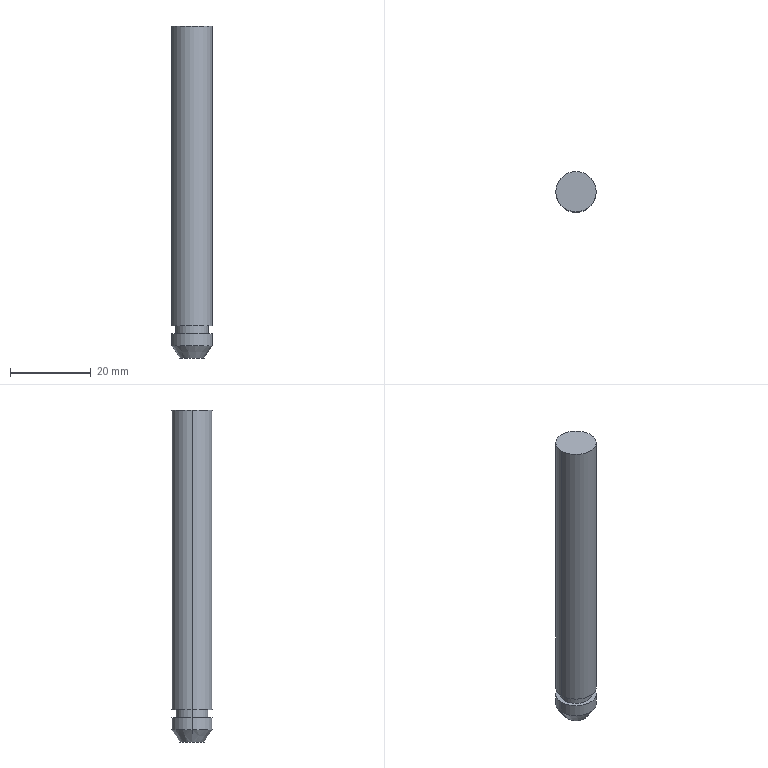Part | SolidWorks | features BaseBody 1 | 1 solid | 12 faces | box 10 x 10 x 82 mm | volume 6302 mm3 | cylinder 6 | plane 4 | cone 2 | commonest cylinder face diameters 10 x4 8 x2
STEP:
#1=CARTESIAN_POINT('',(5.,0.,-74.));
#2=VERTEX_POINT('',#1);
#3=CARTESIAN_POINT('',(-5.,0.,-74.));
#4=VERTEX_POINT('',#3);
#5=CARTESIAN_POINT('',(0.,0.,-74.));
#6=DIRECTION('',(0.,0.,1.));
#7=DIRECTION('',(1.,0.,0.));
#8=AXIS2_PLACEMENT_3D('',#5,#6,#7);
#9=CIRCLE('',#8,5.);
#10=EDGE_CURVE('',#2,#4,#9,.T.);
#11=ORIENTED_EDGE('',*,*,#10,.T.);
#12=CARTESIAN_POINT('',(-5.,0.,0.));
#13=VERTEX_POINT('',#12);
#14=CARTESIAN_POINT('',(-5.,0.,0.));
#15=DIRECTION('',(0.,0.,1.));
#16=VECTOR('',#15,1000.);
#17=LINE('',#14,#16);
#18=EDGE_CURVE('',#4,#13,#17,.T.);
#19=ORIENTED_EDGE('',*,*,#18,.T.);
#20=CARTESIAN_POINT('',(5.,0.,0.));
#21=VERTEX_POINT('',#20);
#22=CARTESIAN_POINT('',(0.,0.,0.));
#23=DIRECTION('',(0.,0.,-1.));
#24=DIRECTION('',(1.,0.,0.));
#25=AXIS2_PLACEMENT_3D('',#22,#23,#24);
#26=CIRCLE('',#25,5.);
#27=EDGE_CURVE('',#13,#21,#26,.T.);
#28=ORIENTED_EDGE('',*,*,#27,.T.);
#29=CARTESIAN_POINT('',(5.,0.,0.));
#30=DIRECTION('',(0.,0.,1.));
#31=VECTOR('',#30,1000.);
#32=LINE('',#29,#31);
#33=EDGE_CURVE('',#2,#21,#32,.T.);
#34=ORIENTED_EDGE('',*,*,#33,.F.);
#35=EDGE_LOOP('',(#11,#19,#28,#34));
#36=FACE_OUTER_BOUND('',#35,.T.);
#37=CARTESIAN_POINT('',(0.,0.,0.));
#38=DIRECTION('',(0.,0.,1.));
#39=DIRECTION('',(1.,0.,0.));
#40=AXIS2_PLACEMENT_3D('',#37,#38,#39);
#41=CYLINDRICAL_SURFACE('',#40,5.);
#42=ADVANCED_FACE('',(#36),#41,.T.);
#43=CARTESIAN_POINT('',(4.,0.,-76.));
#44=VERTEX_POINT('',#43);
#45=CARTESIAN_POINT('',(-4.,0.,-76.));
#46=VERTEX_POINT('',#45);
#47=CARTESIAN_POINT('',(0.,0.,-76.));
#48=DIRECTION('',(0.,0.,1.));
#49=DIRECTION('',(1.,0.,0.));
#50=AXIS2_PLACEMENT_3D('',#47,#48,#49);
#51=CIRCLE('',#50,4.);
#52=EDGE_CURVE('',#44,#46,#51,.T.);
#53=ORIENTED_EDGE('',*,*,#52,.T.);
#54=CARTESIAN_POINT('',(-4.,0.,-74.));
#55=VERTEX_POINT('',#54);
#56=CARTESIAN_POINT('',(-4.,0.,0.));
#57=DIRECTION('',(0.,0.,1.));
#58=VECTOR('',#57,1000.);
#59=LINE('',#56,#58);
#60=EDGE_CURVE('',#46,#55,#59,.T.);
#61=ORIENTED_EDGE('',*,*,#60,.T.);
#62=CARTESIAN_POINT('',(4.,0.,-74.));
#63=VERTEX_POINT('',#62);
#64=CARTESIAN_POINT('',(0.,0.,-74.));
#65=DIRECTION('',(0.,0.,-1.));
#66=DIRECTION('',(1.,0.,0.));
#67=AXIS2_PLACEMENT_3D('',#64,#65,#66);
#68=CIRCLE('',#67,4.);
#69=EDGE_CURVE('',#55,#63,#68,.T.);
#70=ORIENTED_EDGE('',*,*,#69,.T.);
#71=CARTESIAN_POINT('',(4.,0.,0.));
#72=DIRECTION('',(0.,0.,1.));
#73=VECTOR('',#72,1000.);
#74=LINE('',#71,#73);
#75=EDGE_CURVE('',#44,#63,#74,.T.);
#76=ORIENTED_EDGE('',*,*,#75,.F.);
#77=EDGE_LOOP('',(#53,#61,#70,#76));
#78=FACE_OUTER_BOUND('',#77,.T.);
#79=CARTESIAN_POINT('',(0.,0.,0.));
#80=DIRECTION('',(0.,0.,1.));
#81=DIRECTION('',(1.,0.,0.));
#82=AXIS2_PLACEMENT_3D('',#79,#80,#81);
#83=CYLINDRICAL_SURFACE('',#82,4.);
#84=ADVANCED_FACE('',(#78),#83,.T.);
#85=CARTESIAN_POINT('',(5.,0.,-79.));
#86=VERTEX_POINT('',#85);
#87=CARTESIAN_POINT('',(-5.,0.,-79.));
#88=VERTEX_POINT('',#87);
#89=CARTESIAN_POINT('',(0.,0.,-79.));
#90=DIRECTION('',(0.,0.,1.));
#91=DIRECTION('',(1.,0.,0.));
#92=AXIS2_PLACEMENT_3D('',#89,#90,#91);
#93=CIRCLE('',#92,5.);
#94=EDGE_CURVE('',#86,#88,#93,.T.);
#95=ORIENTED_EDGE('',*,*,#94,.T.);
#96=CARTESIAN_POINT('',(-5.,0.,-76.));
#97=VERTEX_POINT('',#96);
#98=CARTESIAN_POINT('',(-5.,0.,0.));
#99=DIRECTION('',(0.,0.,1.));
#100=VECTOR('',#99,1000.);
#101=LINE('',#98,#100);
#102=EDGE_CURVE('',#88,#97,#101,.T.);
#103=ORIENTED_EDGE('',*,*,#102,.T.);
#104=CARTESIAN_POINT('',(5.,0.,-76.));
#105=VERTEX_POINT('',#104);
#106=CARTESIAN_POINT('',(0.,0.,-76.));
#107=DIRECTION('',(0.,0.,-1.));
#108=DIRECTION('',(1.,0.,0.));
#109=AXIS2_PLACEMENT_3D('',#106,#107,#108);
#110=CIRCLE('',#109,5.);
#111=EDGE_CURVE('',#97,#105,#110,.T.);
#112=ORIENTED_EDGE('',*,*,#111,.T.);
#113=CARTESIAN_POINT('',(5.,0.,0.));
#114=DIRECTION('',(0.,0.,1.));
#115=VECTOR('',#114,1000.);
#116=LINE('',#113,#115);
#117=EDGE_CURVE('',#86,#105,#116,.T.);
#118=ORIENTED_EDGE('',*,*,#117,.F.);
#119=EDGE_LOOP('',(#95,#103,#112,#118));
#120=FACE_OUTER_BOUND('',#119,.T.);
#121=CARTESIAN_POINT('',(0.,0.,0.));
#122=DIRECTION('',(0.,0.,1.));
#123=DIRECTION('',(1.,0.,0.));
#124=AXIS2_PLACEMENT_3D('',#121,#122,#123);
#125=CYLINDRICAL_SURFACE('',#124,5.);
#126=ADVANCED_FACE('',(#120),#125,.T.);
#127=CARTESIAN_POINT('',(3.,0.,-82.));
#128=VERTEX_POINT('',#127);
#129=CARTESIAN_POINT('',(-3.,0.,-82.));
#130=VERTEX_POINT('',#129);
#131=CARTESIAN_POINT('',(0.,0.,-82.));
#132=DIRECTION('',(0.,0.,1.));
#133=DIRECTION('',(1.,0.,0.));
#134=AXIS2_PLACEMENT_3D('',#131,#132,#133);
#135=CIRCLE('',#134,3.);
#136=EDGE_CURVE('',#128,#130,#135,.T.);
#137=ORIENTED_EDGE('',*,*,#136,.T.);
#138=CARTESIAN_POINT('',(-5.,0.,-79.));
#139=DIRECTION('',(-0.5547,0.,0.8321));
#140=VECTOR('',#139,1000.);
#141=LINE('',#138,#140);
#142=EDGE_CURVE('',#130,#88,#141,.T.);
#143=ORIENTED_EDGE('',*,*,#142,.T.);
#144=ORIENTED_EDGE('',*,*,#94,.F.);
#145=CARTESIAN_POINT('',(5.,0.,-79.));
#146=DIRECTION('',(0.5547,0.,0.8321));
#147=VECTOR('',#146,1000.);
#148=LINE('',#145,#147);
#149=EDGE_CURVE('',#128,#86,#148,.T.);
#150=ORIENTED_EDGE('',*,*,#149,.F.);
#151=EDGE_LOOP('',(#137,#143,#144,#150));
#152=FACE_OUTER_BOUND('',#151,.T.);
#153=CARTESIAN_POINT('',(0.,0.,-79.));
#154=DIRECTION('',(0.,0.,1.));
#155=DIRECTION('',(1.,0.,0.));
#156=AXIS2_PLACEMENT_3D('',#153,#154,#155);
#157=CONICAL_SURFACE('',#156,5.,0.588);
#158=ADVANCED_FACE('',(#152),#157,.T.);
#159=ORIENTED_EDGE('',*,*,#18,.F.);
#160=CARTESIAN_POINT('',(0.,0.,-74.));
#161=DIRECTION('',(0.,0.,1.));
#162=DIRECTION('',(1.,0.,0.));
#163=AXIS2_PLACEMENT_3D('',#160,#161,#162);
#164=CIRCLE('',#163,5.);
#165=EDGE_CURVE('',#4,#2,#164,.T.);
#166=ORIENTED_EDGE('',*,*,#165,.T.);
#167=ORIENTED_EDGE('',*,*,#33,.T.);
#168=CARTESIAN_POINT('',(0.,0.,0.));
#169=DIRECTION('',(0.,0.,-1.));
#170=DIRECTION('',(1.,0.,0.));
#171=AXIS2_PLACEMENT_3D('',#168,#169,#170);
#172=CIRCLE('',#171,5.);
#173=EDGE_CURVE('',#21,#13,#172,.T.);
#174=ORIENTED_EDGE('',*,*,#173,.T.);
#175=EDGE_LOOP('',(#159,#166,#167,#174));
#176=FACE_OUTER_BOUND('',#175,.T.);
#177=CARTESIAN_POINT('',(0.,0.,0.));
#178=DIRECTION('',(0.,0.,1.));
#179=DIRECTION('',(1.,0.,0.));
#180=AXIS2_PLACEMENT_3D('',#177,#178,#179);
#181=CYLINDRICAL_SURFACE('',#180,5.);
#182=ADVANCED_FACE('',(#176),#181,.T.);
#183=ORIENTED_EDGE('',*,*,#173,.F.);
#184=ORIENTED_EDGE('',*,*,#27,.F.);
#185=EDGE_LOOP('',(#183,#184));
#186=FACE_OUTER_BOUND('',#185,.T.);
#187=CARTESIAN_POINT('',(0.,0.,0.));
#188=DIRECTION('',(0.,0.,-1.));
#189=DIRECTION('',(-1.,0.,0.));
#190=AXIS2_PLACEMENT_3D('',#187,#188,#189);
#191=PLANE('',#190);
#192=ADVANCED_FACE('',(#186),#191,.F.);
#193=ORIENTED_EDGE('',*,*,#10,.F.);
#194=ORIENTED_EDGE('',*,*,#165,.F.);
#195=EDGE_LOOP('',(#193,#194));
#196=FACE_OUTER_BOUND('',#195,.T.);
#197=CARTESIAN_POINT('',(0.,0.,-74.));
#198=DIRECTION('',(0.,0.,-1.));
#199=DIRECTION('',(1.,0.,0.));
#200=AXIS2_PLACEMENT_3D('',#197,#198,#199);
#201=CIRCLE('',#200,4.);
#202=EDGE_CURVE('',#63,#55,#201,.T.);
#203=ORIENTED_EDGE('',*,*,#202,.F.);
#204=ORIENTED_EDGE('',*,*,#69,.F.);
#205=EDGE_LOOP('',(#203,#204));
#206=FACE_BOUND('',#205,.T.);
#207=CARTESIAN_POINT('',(0.,5.,-74.));
#208=DIRECTION('',(0.,0.,1.));
#209=DIRECTION('',(1.,0.,0.));
#210=AXIS2_PLACEMENT_3D('',#207,#208,#209);
#211=PLANE('',#210);
#212=ADVANCED_FACE('',(#196,#206),#211,.F.);
#213=ORIENTED_EDGE('',*,*,#60,.F.);
#214=CARTESIAN_POINT('',(0.,0.,-76.));
#215=DIRECTION('',(0.,0.,1.));
#216=DIRECTION('',(1.,0.,0.));
#217=AXIS2_PLACEMENT_3D('',#214,#215,#216);
#218=CIRCLE('',#217,4.);
#219=EDGE_CURVE('',#46,#44,#218,.T.);
#220=ORIENTED_EDGE('',*,*,#219,.T.);
#221=ORIENTED_EDGE('',*,*,#75,.T.);
#222=ORIENTED_EDGE('',*,*,#202,.T.);
#223=EDGE_LOOP('',(#213,#220,#221,#222));
#224=FACE_OUTER_BOUND('',#223,.T.);
#225=CARTESIAN_POINT('',(0.,0.,0.));
#226=DIRECTION('',(0.,0.,1.));
#227=DIRECTION('',(1.,0.,0.));
#228=AXIS2_PLACEMENT_3D('',#225,#226,#227);
#229=CYLINDRICAL_SURFACE('',#228,4.);
#230=ADVANCED_FACE('',(#224),#229,.T.);
#231=ORIENTED_EDGE('',*,*,#52,.F.);
#232=ORIENTED_EDGE('',*,*,#219,.F.);
#233=EDGE_LOOP('',(#231,#232));
#234=FACE_BOUND('',#233,.T.);
#235=CARTESIAN_POINT('',(0.,0.,-76.));
#236=DIRECTION('',(0.,0.,-1.));
#237=DIRECTION('',(1.,0.,0.));
#238=AXIS2_PLACEMENT_3D('',#235,#236,#237);
#239=CIRCLE('',#238,5.);
#240=EDGE_CURVE('',#105,#97,#239,.T.);
#241=ORIENTED_EDGE('',*,*,#240,.F.);
#242=ORIENTED_EDGE('',*,*,#111,.F.);
#243=EDGE_LOOP('',(#241,#242));
#244=FACE_OUTER_BOUND('',#243,.T.);
#245=CARTESIAN_POINT('',(0.,4.,-76.));
#246=DIRECTION('',(0.,0.,-1.));
#247=DIRECTION('',(-1.,0.,0.));
#248=AXIS2_PLACEMENT_3D('',#245,#246,#247);
#249=PLANE('',#248);
#250=ADVANCED_FACE('',(#234,#244),#249,.F.);
#251=ORIENTED_EDGE('',*,*,#102,.F.);
#252=CARTESIAN_POINT('',(0.,0.,-79.));
#253=DIRECTION('',(0.,0.,1.));
#254=DIRECTION('',(1.,0.,0.));
#255=AXIS2_PLACEMENT_3D('',#252,#253,#254);
#256=CIRCLE('',#255,5.);
#257=EDGE_CURVE('',#88,#86,#256,.T.);
#258=ORIENTED_EDGE('',*,*,#257,.T.);
#259=ORIENTED_EDGE('',*,*,#117,.T.);
#260=ORIENTED_EDGE('',*,*,#240,.T.);
#261=EDGE_LOOP('',(#251,#258,#259,#260));
#262=FACE_OUTER_BOUND('',#261,.T.);
#263=CARTESIAN_POINT('',(0.,0.,0.));
#264=DIRECTION('',(0.,0.,1.));
#265=DIRECTION('',(1.,0.,0.));
#266=AXIS2_PLACEMENT_3D('',#263,#264,#265);
#267=CYLINDRICAL_SURFACE('',#266,5.);
#268=ADVANCED_FACE('',(#262),#267,.T.);
#269=ORIENTED_EDGE('',*,*,#142,.F.);
#270=CARTESIAN_POINT('',(0.,0.,-82.));
#271=DIRECTION('',(0.,0.,1.));
#272=DIRECTION('',(1.,0.,0.));
#273=AXIS2_PLACEMENT_3D('',#270,#271,#272);
#274=CIRCLE('',#273,3.);
#275=EDGE_CURVE('',#130,#128,#274,.T.);
#276=ORIENTED_EDGE('',*,*,#275,.T.);
#277=ORIENTED_EDGE('',*,*,#149,.T.);
#278=ORIENTED_EDGE('',*,*,#257,.F.);
#279=EDGE_LOOP('',(#269,#276,#277,#278));
#280=FACE_OUTER_BOUND('',#279,.T.);
#281=CARTESIAN_POINT('',(0.,0.,-79.));
#282=DIRECTION('',(0.,0.,1.));
#283=DIRECTION('',(1.,0.,0.));
#284=AXIS2_PLACEMENT_3D('',#281,#282,#283);
#285=CONICAL_SURFACE('',#284,5.,0.588);
#286=ADVANCED_FACE('',(#280),#285,.T.);
#287=ORIENTED_EDGE('',*,*,#136,.F.);
#288=ORIENTED_EDGE('',*,*,#275,.F.);
#289=EDGE_LOOP('',(#287,#288));
#290=FACE_OUTER_BOUND('',#289,.T.);
#291=CARTESIAN_POINT('',(0.,3.,-82.));
#292=DIRECTION('',(0.,0.,1.));
#293=DIRECTION('',(1.,0.,0.));
#294=AXIS2_PLACEMENT_3D('',#291,#292,#293);
#295=PLANE('',#294);
#296=ADVANCED_FACE('',(#290),#295,.F.);
#297=CLOSED_SHELL('',(#42,#84,#126,#158,#182,#192,#212,#230,#250,#268,#286,#296));
#298=MANIFOLD_SOLID_BREP('',#297);
#299=CARTESIAN_POINT('',(0.,0.,0.));
#300=DIRECTION('',(0.,0.,1.));
#301=DIRECTION('',(1.,0.,0.));
#302=AXIS2_PLACEMENT_3D('',#299,#300,#301);
#303=(LENGTH_UNIT()NAMED_UNIT(*)SI_UNIT(.MILLI.,.METRE.));
#304=UNCERTAINTY_MEASURE_WITH_UNIT(LENGTH_MEASURE(0.00001),#303,'','');
#305=(NAMED_UNIT(*)PLANE_ANGLE_UNIT()SI_UNIT($,.RADIAN.));
#306=(NAMED_UNIT(*)SI_UNIT($,.STERADIAN.)SOLID_ANGLE_UNIT());
#307=(GEOMETRIC_REPRESENTATION_CONTEXT(3)GLOBAL_UNCERTAINTY_ASSIGNED_CONTEXT((#304))GLOBAL_UNIT_ASSIGNED_CONTEXT((#303,#305,#306))REPRESENTATION_CONTEXT('',''));
#308=ADVANCED_BREP_SHAPE_REPRESENTATION('',(#298,#302),#307);